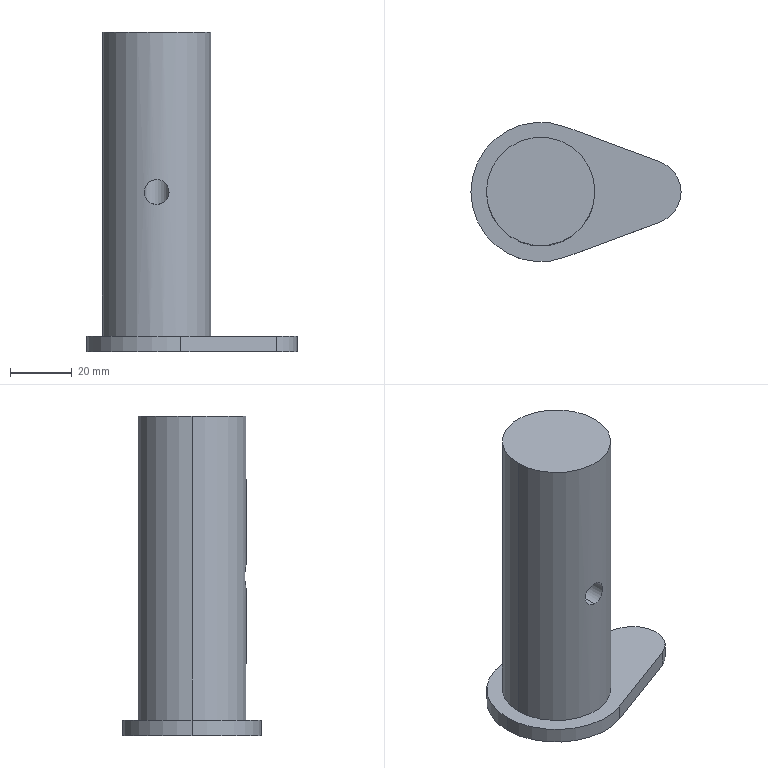Part | SolidWorks | features ICE 3, Extrusion 1 | 1 solid | 16 faces | box 67.801 x 45 x 103 mm | volume 100967 mm3 | cylinder 10 | plane 6 | commonest cylinder face diameters 8 x5 35 x2 45 x2 20.602 x1
STEP:
#1=CARTESIAN_POINT('',(0.,-17.5,47.5));
#2=VERTEX_POINT('',#1);
#3=CARTESIAN_POINT('',(0.,-17.5,55.5));
#4=VERTEX_POINT('',#3);
#5=CARTESIAN_POINT('',(0.,-17.5,47.5));
#6=CARTESIAN_POINT('',(-0.2615,-17.5,47.5));
#7=CARTESIAN_POINT('',(-0.522,-17.494,47.525));
#8=CARTESIAN_POINT('',(-1.041,-17.471,47.629));
#9=CARTESIAN_POINT('',(-1.292,-17.454,47.705));
#10=CARTESIAN_POINT('',(-1.773,-17.412,47.905));
#11=CARTESIAN_POINT('',(-2.007,-17.386,48.03));
#12=CARTESIAN_POINT('',(-2.442,-17.33,48.321));
#13=CARTESIAN_POINT('',(-2.643,-17.3,48.486));
#14=CARTESIAN_POINT('',(-3.012,-17.24,48.854));
#15=CARTESIAN_POINT('',(-3.18,-17.209,49.059));
#16=CARTESIAN_POINT('',(-3.469,-17.153,49.492));
#17=CARTESIAN_POINT('',(-3.592,-17.128,49.721));
#18=CARTESIAN_POINT('',(-3.794,-17.084,50.207));
#19=CARTESIAN_POINT('',(-3.871,-17.067,50.459));
#20=CARTESIAN_POINT('',(-3.973,-17.043,50.971));
#21=CARTESIAN_POINT('',(-4.,-17.037,51.234));
#22=CARTESIAN_POINT('',(-4.,-17.037,51.762));
#23=CARTESIAN_POINT('',(-3.974,-17.043,52.023));
#24=CARTESIAN_POINT('',(-3.872,-17.066,52.536));
#25=CARTESIAN_POINT('',(-3.795,-17.084,52.791));
#26=CARTESIAN_POINT('',(-3.595,-17.127,53.274));
#27=CARTESIAN_POINT('',(-3.472,-17.153,53.503));
#28=CARTESIAN_POINT('',(-3.181,-17.209,53.939));
#29=CARTESIAN_POINT('',(-3.014,-17.24,54.143));
#30=CARTESIAN_POINT('',(-2.647,-17.3,54.51));
#31=CARTESIAN_POINT('',(-2.444,-17.33,54.677));
#32=CARTESIAN_POINT('',(-2.008,-17.386,54.97));
#33=CARTESIAN_POINT('',(-1.778,-17.411,55.093));
#34=CARTESIAN_POINT('',(-1.297,-17.454,55.293));
#35=CARTESIAN_POINT('',(-1.042,-17.471,55.371));
#36=CARTESIAN_POINT('',(-0.5267,-17.494,55.474));
#37=CARTESIAN_POINT('',(-0.2652,-17.5,55.5));
#38=CARTESIAN_POINT('',(0.,-17.5,55.5));
#39=B_SPLINE_CURVE_WITH_KNOTS('',3,(#5,#6,#7,#8,#9,#10,#11,#12,#13,#14,#15,#16,#17,#18,#19,#20,#21,#22,#23,#24,#25,#26,#27,#28,#29,#30,#31,#32,#33,#34,#35,#36,#37,#38),.UNSPECIFIED.,.F.,.F.,(4,2,2,2,2,2,2,2,2,2,2,2,2,2,2,2,4),(0.01255,0.01333,0.01412,0.0149,0.01568,0.01647,0.01725,0.01804,0.01882,0.0196,0.02039,0.02117,0.02196,0.02274,0.02352,0.02431,0.02509),.UNSPECIFIED.);
#40=EDGE_CURVE('',#2,#4,#39,.T.);
#41=ORIENTED_EDGE('',*,*,#40,.F.);
#42=CARTESIAN_POINT('',(0.,-4.,47.5));
#43=VERTEX_POINT('',#42);
#44=CARTESIAN_POINT('',(0.,-70.,47.5));
#45=DIRECTION('',(0.,1.,0.));
#46=VECTOR('',#45,1000.);
#47=LINE('',#44,#46);
#48=EDGE_CURVE('',#2,#43,#47,.T.);
#49=ORIENTED_EDGE('',*,*,#48,.T.);
#50=CARTESIAN_POINT('',(-4.,0.,51.5));
#51=VERTEX_POINT('',#50);
#52=CARTESIAN_POINT('',(-4.,0.,51.5));
#53=CARTESIAN_POINT('',(-4.,-2.343,49.157));
#54=CARTESIAN_POINT('',(-2.343,-4.,47.5));
#55=CARTESIAN_POINT('',(0.,-4.,47.5));
#56=(BOUNDED_CURVE()B_SPLINE_CURVE(3,(#52,#53,#54,#55),.UNSPECIFIED.,.F.,.F.)B_SPLINE_CURVE_WITH_KNOTS((4,4),(4.712,6.283),.UNSPECIFIED.)CURVE()GEOMETRIC_REPRESENTATION_ITEM()RATIONAL_B_SPLINE_CURVE((1.,0.8047,0.8047,1.))REPRESENTATION_ITEM(''));
#57=EDGE_CURVE('',#51,#43,#56,.T.);
#58=ORIENTED_EDGE('',*,*,#57,.F.);
#59=CARTESIAN_POINT('',(0.,-4.,55.5));
#60=VERTEX_POINT('',#59);
#61=CARTESIAN_POINT('',(0.,-4.,55.5));
#62=CARTESIAN_POINT('',(-2.343,-4.,55.5));
#63=CARTESIAN_POINT('',(-4.,-2.343,53.843));
#64=CARTESIAN_POINT('',(-4.,0.,51.5));
#65=(BOUNDED_CURVE()B_SPLINE_CURVE(3,(#61,#62,#63,#64),.UNSPECIFIED.,.F.,.T.)B_SPLINE_CURVE_WITH_KNOTS((4,4),(3.142,4.712),.UNSPECIFIED.)CURVE()GEOMETRIC_REPRESENTATION_ITEM()RATIONAL_B_SPLINE_CURVE((1.,0.8047,0.8047,1.))REPRESENTATION_ITEM(''));
#66=EDGE_CURVE('',#60,#51,#65,.T.);
#67=ORIENTED_EDGE('',*,*,#66,.F.);
#68=CARTESIAN_POINT('',(0.,-70.,55.5));
#69=DIRECTION('',(0.,1.,0.));
#70=VECTOR('',#69,1000.);
#71=LINE('',#68,#70);
#72=EDGE_CURVE('',#4,#60,#71,.T.);
#73=ORIENTED_EDGE('',*,*,#72,.F.);
#74=EDGE_LOOP('',(#41,#49,#58,#67,#73));
#75=FACE_OUTER_BOUND('',#74,.T.);
#76=CARTESIAN_POINT('',(0.,-70.,51.5));
#77=DIRECTION('',(0.,1.,0.));
#78=DIRECTION('',(0.,0.,1.));
#79=AXIS2_PLACEMENT_3D('',#76,#77,#78);
#80=CYLINDRICAL_SURFACE('',#79,4.);
#81=ADVANCED_FACE('',(#75),#80,.F.);
#82=CARTESIAN_POINT('',(4.,0.,70.));
#83=VERTEX_POINT('',#82);
#84=CARTESIAN_POINT('',(-4.,0.,70.));
#85=VERTEX_POINT('',#84);
#86=CARTESIAN_POINT('',(0.,0.,70.));
#87=DIRECTION('',(0.,0.,-1.));
#88=DIRECTION('',(-1.,0.,0.));
#89=AXIS2_PLACEMENT_3D('',#86,#87,#88);
#90=CIRCLE('',#89,4.);
#91=EDGE_CURVE('',#83,#85,#90,.T.);
#92=ORIENTED_EDGE('',*,*,#91,.F.);
#93=CARTESIAN_POINT('',(4.,0.,51.5));
#94=VERTEX_POINT('',#93);
#95=CARTESIAN_POINT('',(4.,0.,70.));
#96=DIRECTION('',(0.,0.,-1.));
#97=VECTOR('',#96,1000.);
#98=LINE('',#95,#97);
#99=EDGE_CURVE('',#83,#94,#98,.T.);
#100=ORIENTED_EDGE('',*,*,#99,.T.);
#101=CARTESIAN_POINT('',(4.,0.,51.5));
#102=CARTESIAN_POINT('',(4.,-2.343,53.843));
#103=CARTESIAN_POINT('',(2.343,-4.,55.5));
#104=CARTESIAN_POINT('',(0.,-4.,55.5));
#105=(BOUNDED_CURVE()B_SPLINE_CURVE(3,(#101,#102,#103,#104),.UNSPECIFIED.,.F.,.T.)B_SPLINE_CURVE_WITH_KNOTS((4,4),(1.571,3.142),.UNSPECIFIED.)CURVE()GEOMETRIC_REPRESENTATION_ITEM()RATIONAL_B_SPLINE_CURVE((1.,0.8047,0.8047,1.))REPRESENTATION_ITEM(''));
#106=EDGE_CURVE('',#94,#60,#105,.T.);
#107=ORIENTED_EDGE('',*,*,#106,.T.);
#108=ORIENTED_EDGE('',*,*,#66,.T.);
#109=CARTESIAN_POINT('',(-4.,0.,70.));
#110=DIRECTION('',(0.,0.,-1.));
#111=VECTOR('',#110,1000.);
#112=LINE('',#109,#111);
#113=EDGE_CURVE('',#85,#51,#112,.T.);
#114=ORIENTED_EDGE('',*,*,#113,.F.);
#115=EDGE_LOOP('',(#92,#100,#107,#108,#114));
#116=FACE_OUTER_BOUND('',#115,.T.);
#117=CARTESIAN_POINT('',(0.,0.,70.));
#118=DIRECTION('',(0.,0.,-1.));
#119=DIRECTION('',(-1.,0.,0.));
#120=AXIS2_PLACEMENT_3D('',#117,#118,#119);
#121=CYLINDRICAL_SURFACE('',#120,4.);
#122=ADVANCED_FACE('',(#116),#121,.F.);
#123=ORIENTED_EDGE('',*,*,#57,.T.);
#124=CARTESIAN_POINT('',(0.,-4.,47.5));
#125=CARTESIAN_POINT('',(2.343,-4.,47.5));
#126=CARTESIAN_POINT('',(4.,-2.343,49.157));
#127=CARTESIAN_POINT('',(4.,0.,51.5));
#128=(BOUNDED_CURVE()B_SPLINE_CURVE(3,(#124,#125,#126,#127),.UNSPECIFIED.,.F.,.F.)B_SPLINE_CURVE_WITH_KNOTS((4,4),(0.,1.571),.UNSPECIFIED.)CURVE()GEOMETRIC_REPRESENTATION_ITEM()RATIONAL_B_SPLINE_CURVE((1.,0.8047,0.8047,1.))REPRESENTATION_ITEM(''));
#129=EDGE_CURVE('',#43,#94,#128,.T.);
#130=ORIENTED_EDGE('',*,*,#129,.T.);
#131=CARTESIAN_POINT('',(4.,0.,0.));
#132=VERTEX_POINT('',#131);
#133=CARTESIAN_POINT('',(4.,0.,70.));
#134=DIRECTION('',(0.,0.,-1.));
#135=VECTOR('',#134,1000.);
#136=LINE('',#133,#135);
#137=EDGE_CURVE('',#94,#132,#136,.T.);
#138=ORIENTED_EDGE('',*,*,#137,.T.);
#139=CARTESIAN_POINT('',(-4.,0.,0.));
#140=VERTEX_POINT('',#139);
#141=CARTESIAN_POINT('',(0.,0.,0.));
#142=DIRECTION('',(0.,0.,-1.));
#143=DIRECTION('',(-1.,0.,0.));
#144=AXIS2_PLACEMENT_3D('',#141,#142,#143);
#145=CIRCLE('',#144,4.);
#146=EDGE_CURVE('',#132,#140,#145,.T.);
#147=ORIENTED_EDGE('',*,*,#146,.T.);
#148=CARTESIAN_POINT('',(-4.,0.,70.));
#149=DIRECTION('',(0.,0.,-1.));
#150=VECTOR('',#149,1000.);
#151=LINE('',#148,#150);
#152=EDGE_CURVE('',#51,#140,#151,.T.);
#153=ORIENTED_EDGE('',*,*,#152,.F.);
#154=EDGE_LOOP('',(#123,#130,#138,#147,#153));
#155=FACE_OUTER_BOUND('',#154,.T.);
#156=CARTESIAN_POINT('',(0.,0.,70.));
#157=DIRECTION('',(0.,0.,-1.));
#158=DIRECTION('',(-1.,0.,0.));
#159=AXIS2_PLACEMENT_3D('',#156,#157,#158);
#160=CYLINDRICAL_SURFACE('',#159,4.);
#161=ADVANCED_FACE('',(#155),#160,.F.);
#162=CARTESIAN_POINT('',(7.842,-21.089,5.));
#163=VERTEX_POINT('',#162);
#164=CARTESIAN_POINT('',(-22.5,0.,5.));
#165=VERTEX_POINT('',#164);
#166=CARTESIAN_POINT('',(0.,0.,5.));
#167=DIRECTION('',(0.,0.,-1.));
#168=DIRECTION('',(-1.,0.,0.));
#169=AXIS2_PLACEMENT_3D('',#166,#167,#168);
#170=CIRCLE('',#169,22.5);
#171=EDGE_CURVE('',#163,#165,#170,.T.);
#172=ORIENTED_EDGE('',*,*,#171,.T.);
#173=CARTESIAN_POINT('',(-22.5,0.,0.));
#174=VERTEX_POINT('',#173);
#175=CARTESIAN_POINT('',(-22.5,0.,5.));
#176=DIRECTION('',(0.,0.,-1.));
#177=VECTOR('',#176,1000.);
#178=LINE('',#175,#177);
#179=EDGE_CURVE('',#165,#174,#178,.T.);
#180=ORIENTED_EDGE('',*,*,#179,.T.);
#181=CARTESIAN_POINT('',(7.842,-21.089,0.));
#182=VERTEX_POINT('',#181);
#183=CARTESIAN_POINT('',(0.,0.,0.));
#184=DIRECTION('',(0.,0.,-1.));
#185=DIRECTION('',(-1.,0.,0.));
#186=AXIS2_PLACEMENT_3D('',#183,#184,#185);
#187=CIRCLE('',#186,22.5);
#188=EDGE_CURVE('',#182,#174,#187,.T.);
#189=ORIENTED_EDGE('',*,*,#188,.F.);
#190=CARTESIAN_POINT('',(7.842,-21.089,5.));
#191=DIRECTION('',(0.,0.,-1.));
#192=VECTOR('',#191,1000.);
#193=LINE('',#190,#192);
#194=EDGE_CURVE('',#163,#182,#193,.T.);
#195=ORIENTED_EDGE('',*,*,#194,.F.);
#196=EDGE_LOOP('',(#172,#180,#189,#195));
#197=FACE_OUTER_BOUND('',#196,.T.);
#198=CARTESIAN_POINT('',(0.,0.,5.));
#199=DIRECTION('',(0.,0.,-1.));
#200=DIRECTION('',(-1.,0.,0.));
#201=AXIS2_PLACEMENT_3D('',#198,#199,#200);
#202=CYLINDRICAL_SURFACE('',#201,22.5);
#203=ADVANCED_FACE('',(#197),#202,.T.);
#204=CARTESIAN_POINT('',(17.5,0.,103.));
#205=VERTEX_POINT('',#204);
#206=CARTESIAN_POINT('',(-17.5,0.,103.));
#207=VERTEX_POINT('',#206);
#208=CARTESIAN_POINT('',(0.,0.,103.));
#209=DIRECTION('',(0.,0.,1.));
#210=DIRECTION('',(1.,0.,0.));
#211=AXIS2_PLACEMENT_3D('',#208,#209,#210);
#212=CIRCLE('',#211,17.5);
#213=EDGE_CURVE('',#205,#207,#212,.T.);
#214=ORIENTED_EDGE('',*,*,#213,.F.);
#215=CARTESIAN_POINT('',(17.5,0.,5.));
#216=VERTEX_POINT('',#215);
#217=CARTESIAN_POINT('',(17.5,0.,103.));
#218=DIRECTION('',(0.,0.,-1.));
#219=VECTOR('',#218,1000.);
#220=LINE('',#217,#219);
#221=EDGE_CURVE('',#205,#216,#220,.T.);
#222=ORIENTED_EDGE('',*,*,#221,.T.);
#223=CARTESIAN_POINT('',(-17.5,0.,5.));
#224=VERTEX_POINT('',#223);
#225=CARTESIAN_POINT('',(0.,0.,5.));
#226=DIRECTION('',(0.,0.,-1.));
#227=DIRECTION('',(-1.,0.,0.));
#228=AXIS2_PLACEMENT_3D('',#225,#226,#227);
#229=CIRCLE('',#228,17.5);
#230=EDGE_CURVE('',#224,#216,#229,.T.);
#231=ORIENTED_EDGE('',*,*,#230,.F.);
#232=CARTESIAN_POINT('',(-17.5,0.,103.));
#233=DIRECTION('',(0.,0.,-1.));
#234=VECTOR('',#233,1000.);
#235=LINE('',#232,#234);
#236=EDGE_CURVE('',#207,#224,#235,.T.);
#237=ORIENTED_EDGE('',*,*,#236,.F.);
#238=EDGE_LOOP('',(#214,#222,#231,#237));
#239=FACE_OUTER_BOUND('',#238,.T.);
#240=CARTESIAN_POINT('',(0.,0.,103.));
#241=DIRECTION('',(0.,0.,-1.));
#242=DIRECTION('',(-1.,0.,0.));
#243=AXIS2_PLACEMENT_3D('',#240,#241,#242);
#244=CYLINDRICAL_SURFACE('',#243,17.5);
#245=ADVANCED_FACE('',(#239),#244,.T.);
#246=ORIENTED_EDGE('',*,*,#221,.F.);
#247=CARTESIAN_POINT('',(0.,0.,103.));
#248=DIRECTION('',(0.,0.,1.));
#249=DIRECTION('',(1.,0.,0.));
#250=AXIS2_PLACEMENT_3D('',#247,#248,#249);
#251=CIRCLE('',#250,17.5);
#252=EDGE_CURVE('',#207,#205,#251,.T.);
#253=ORIENTED_EDGE('',*,*,#252,.F.);
#254=ORIENTED_EDGE('',*,*,#236,.T.);
#255=CARTESIAN_POINT('',(0.,0.,5.));
#256=DIRECTION('',(0.,0.,-1.));
#257=DIRECTION('',(-1.,0.,0.));
#258=AXIS2_PLACEMENT_3D('',#255,#256,#257);
#259=CIRCLE('',#258,17.5);
#260=EDGE_CURVE('',#216,#224,#259,.T.);
#261=ORIENTED_EDGE('',*,*,#260,.F.);
#262=EDGE_LOOP('',(#246,#253,#254,#261));
#263=FACE_OUTER_BOUND('',#262,.T.);
#264=CARTESIAN_POINT('',(0.,-17.5,55.5));
#265=CARTESIAN_POINT('',(0.2652,-17.5,55.5));
#266=CARTESIAN_POINT('',(0.5259,-17.494,55.474));
#267=CARTESIAN_POINT('',(1.038,-17.471,55.372));
#268=CARTESIAN_POINT('',(1.293,-17.454,55.294));
#269=CARTESIAN_POINT('',(1.777,-17.411,55.093));
#270=CARTESIAN_POINT('',(2.006,-17.386,54.97));
#271=CARTESIAN_POINT('',(2.441,-17.33,54.68));
#272=CARTESIAN_POINT('',(2.645,-17.3,54.512));
#273=CARTESIAN_POINT('',(3.013,-17.24,54.144));
#274=CARTESIAN_POINT('',(3.178,-17.21,53.943));
#275=CARTESIAN_POINT('',(3.471,-17.153,53.506));
#276=CARTESIAN_POINT('',(3.594,-17.127,53.274));
#277=CARTESIAN_POINT('',(3.794,-17.084,52.793));
#278=CARTESIAN_POINT('',(3.871,-17.067,52.54));
#279=CARTESIAN_POINT('',(3.974,-17.043,52.024));
#280=CARTESIAN_POINT('',(4.,-17.037,51.763));
#281=CARTESIAN_POINT('',(4.,-17.037,51.24));
#282=CARTESIAN_POINT('',(3.974,-17.043,50.974));
#283=CARTESIAN_POINT('',(3.871,-17.067,50.46));
#284=CARTESIAN_POINT('',(3.795,-17.084,50.21));
#285=CARTESIAN_POINT('',(3.594,-17.127,49.725));
#286=CARTESIAN_POINT('',(3.469,-17.153,49.492));
#287=CARTESIAN_POINT('',(3.18,-17.209,49.06));
#288=CARTESIAN_POINT('',(3.014,-17.24,48.857));
#289=CARTESIAN_POINT('',(2.642,-17.3,48.486));
#290=CARTESIAN_POINT('',(2.441,-17.33,48.321));
#291=CARTESIAN_POINT('',(2.009,-17.386,48.031));
#292=CARTESIAN_POINT('',(1.774,-17.411,47.906));
#293=CARTESIAN_POINT('',(1.291,-17.454,47.705));
#294=CARTESIAN_POINT('',(1.042,-17.471,47.629));
#295=CARTESIAN_POINT('',(0.5271,-17.494,47.526));
#296=CARTESIAN_POINT('',(0.2616,-17.5,47.5));
#297=CARTESIAN_POINT('',(0.,-17.5,47.5));
#298=B_SPLINE_CURVE_WITH_KNOTS('',3,(#264,#265,#266,#267,#268,#269,#270,#271,#272,#273,#274,#275,#276,#277,#278,#279,#280,#281,#282,#283,#284,#285,#286,#287,#288,#289,#290,#291,#292,#293,#294,#295,#296,#297),.UNSPECIFIED.,.F.,.F.,(4,2,2,2,2,2,2,2,2,2,2,2,2,2,2,2,4),(0.,0.0007842,0.001568,0.002353,0.003137,0.003921,0.004705,0.005489,0.006274,0.007058,0.007842,0.008626,0.009411,0.01019,0.01098,0.01176,0.01255),.UNSPECIFIED.);
#299=EDGE_CURVE('',#4,#2,#298,.T.);
#300=ORIENTED_EDGE('',*,*,#299,.T.);
#301=ORIENTED_EDGE('',*,*,#40,.T.);
#302=EDGE_LOOP('',(#300,#301));
#303=FACE_BOUND('',#302,.T.);
#304=CARTESIAN_POINT('',(0.,0.,103.));
#305=DIRECTION('',(0.,0.,-1.));
#306=DIRECTION('',(-1.,0.,0.));
#307=AXIS2_PLACEMENT_3D('',#304,#305,#306);
#308=CYLINDRICAL_SURFACE('',#307,17.5);
#309=ADVANCED_FACE('',(#263,#303),#308,.T.);
#310=ORIENTED_EDGE('',*,*,#252,.T.);
#311=ORIENTED_EDGE('',*,*,#213,.T.);
#312=EDGE_LOOP('',(#310,#311));
#313=FACE_OUTER_BOUND('',#312,.T.);
#314=CARTESIAN_POINT('',(0.,0.,103.));
#315=DIRECTION('',(0.,0.,1.));
#316=DIRECTION('',(1.,0.,0.));
#317=AXIS2_PLACEMENT_3D('',#314,#315,#316);
#318=PLANE('',#317);
#319=ADVANCED_FACE('',(#313),#318,.T.);
#320=CARTESIAN_POINT('',(38.59,-9.655,5.));
#321=VERTEX_POINT('',#320);
#322=CARTESIAN_POINT('',(7.842,-21.089,5.));
#323=DIRECTION('',(-0.9373,-0.3485,0.));
#324=VECTOR('',#323,1000.);
#325=LINE('',#322,#324);
#326=EDGE_CURVE('',#321,#163,#325,.T.);
#327=ORIENTED_EDGE('',*,*,#326,.F.);
#328=CARTESIAN_POINT('',(38.59,9.655,5.));
#329=VERTEX_POINT('',#328);
#330=CARTESIAN_POINT('',(35.,0.,5.));
#331=DIRECTION('',(0.,0.,-1.));
#332=DIRECTION('',(-1.,0.,0.));
#333=AXIS2_PLACEMENT_3D('',#330,#331,#332);
#334=CIRCLE('',#333,10.301);
#335=EDGE_CURVE('',#329,#321,#334,.T.);
#336=ORIENTED_EDGE('',*,*,#335,.F.);
#337=CARTESIAN_POINT('',(7.842,21.089,5.));
#338=VERTEX_POINT('',#337);
#339=CARTESIAN_POINT('',(7.842,21.089,5.));
#340=DIRECTION('',(-0.9373,0.3485,0.));
#341=VECTOR('',#340,1000.);
#342=LINE('',#339,#341);
#343=EDGE_CURVE('',#329,#338,#342,.T.);
#344=ORIENTED_EDGE('',*,*,#343,.T.);
#345=CARTESIAN_POINT('',(0.,0.,5.));
#346=DIRECTION('',(0.,0.,-1.));
#347=DIRECTION('',(-1.,0.,0.));
#348=AXIS2_PLACEMENT_3D('',#345,#346,#347);
#349=CIRCLE('',#348,22.5);
#350=EDGE_CURVE('',#165,#338,#349,.T.);
#351=ORIENTED_EDGE('',*,*,#350,.F.);
#352=ORIENTED_EDGE('',*,*,#171,.F.);
#353=EDGE_LOOP('',(#327,#336,#344,#351,#352));
#354=FACE_OUTER_BOUND('',#353,.T.);
#355=ORIENTED_EDGE('',*,*,#230,.T.);
#356=ORIENTED_EDGE('',*,*,#260,.T.);
#357=EDGE_LOOP('',(#355,#356));
#358=FACE_BOUND('',#357,.T.);
#359=CARTESIAN_POINT('',(0.,0.,5.));
#360=DIRECTION('',(0.,0.,-1.));
#361=DIRECTION('',(-1.,0.,0.));
#362=AXIS2_PLACEMENT_3D('',#359,#360,#361);
#363=PLANE('',#362);
#364=ADVANCED_FACE('',(#354,#358),#363,.F.);
#365=CARTESIAN_POINT('',(38.59,-9.655,0.));
#366=VERTEX_POINT('',#365);
#367=CARTESIAN_POINT('',(7.842,-21.089,0.));
#368=DIRECTION('',(-0.9373,-0.3485,0.));
#369=VECTOR('',#368,1000.);
#370=LINE('',#367,#369);
#371=EDGE_CURVE('',#366,#182,#370,.T.);
#372=ORIENTED_EDGE('',*,*,#371,.F.);
#373=CARTESIAN_POINT('',(38.59,-9.655,5.));
#374=DIRECTION('',(0.,0.,-1.));
#375=VECTOR('',#374,1000.);
#376=LINE('',#373,#375);
#377=EDGE_CURVE('',#321,#366,#376,.T.);
#378=ORIENTED_EDGE('',*,*,#377,.F.);
#379=ORIENTED_EDGE('',*,*,#326,.T.);
#380=ORIENTED_EDGE('',*,*,#194,.T.);
#381=EDGE_LOOP('',(#372,#378,#379,#380));
#382=FACE_OUTER_BOUND('',#381,.T.);
#383=CARTESIAN_POINT('',(7.842,-21.089,5.));
#384=DIRECTION('',(0.3485,-0.9373,0.));
#385=DIRECTION('',(0.9373,0.3485,0.));
#386=AXIS2_PLACEMENT_3D('',#383,#384,#385);
#387=PLANE('',#386);
#388=ADVANCED_FACE('',(#382),#387,.T.);
#389=CARTESIAN_POINT('',(38.59,9.655,0.));
#390=VERTEX_POINT('',#389);
#391=CARTESIAN_POINT('',(35.,0.,0.));
#392=DIRECTION('',(0.,0.,-1.));
#393=DIRECTION('',(-1.,0.,0.));
#394=AXIS2_PLACEMENT_3D('',#391,#392,#393);
#395=CIRCLE('',#394,10.301);
#396=EDGE_CURVE('',#390,#366,#395,.T.);
#397=ORIENTED_EDGE('',*,*,#396,.F.);
#398=CARTESIAN_POINT('',(38.59,9.655,5.));
#399=DIRECTION('',(0.,0.,-1.));
#400=VECTOR('',#399,1000.);
#401=LINE('',#398,#400);
#402=EDGE_CURVE('',#329,#390,#401,.T.);
#403=ORIENTED_EDGE('',*,*,#402,.F.);
#404=ORIENTED_EDGE('',*,*,#335,.T.);
#405=ORIENTED_EDGE('',*,*,#377,.T.);
#406=EDGE_LOOP('',(#397,#403,#404,#405));
#407=FACE_OUTER_BOUND('',#406,.T.);
#408=CARTESIAN_POINT('',(35.,0.,5.));
#409=DIRECTION('',(0.,0.,-1.));
#410=DIRECTION('',(-1.,0.,0.));
#411=AXIS2_PLACEMENT_3D('',#408,#409,#410);
#412=CYLINDRICAL_SURFACE('',#411,10.301);
#413=ADVANCED_FACE('',(#407),#412,.T.);
#414=CARTESIAN_POINT('',(7.842,21.089,0.));
#415=VERTEX_POINT('',#414);
#416=CARTESIAN_POINT('',(7.842,21.089,0.));
#417=DIRECTION('',(-0.9373,0.3485,0.));
#418=VECTOR('',#417,1000.);
#419=LINE('',#416,#418);
#420=EDGE_CURVE('',#390,#415,#419,.T.);
#421=ORIENTED_EDGE('',*,*,#420,.T.);
#422=CARTESIAN_POINT('',(7.842,21.089,5.));
#423=DIRECTION('',(0.,0.,-1.));
#424=VECTOR('',#423,1000.);
#425=LINE('',#422,#424);
#426=EDGE_CURVE('',#338,#415,#425,.T.);
#427=ORIENTED_EDGE('',*,*,#426,.F.);
#428=ORIENTED_EDGE('',*,*,#343,.F.);
#429=ORIENTED_EDGE('',*,*,#402,.T.);
#430=EDGE_LOOP('',(#421,#427,#428,#429));
#431=FACE_OUTER_BOUND('',#430,.T.);
#432=CARTESIAN_POINT('',(7.842,21.089,5.));
#433=DIRECTION('',(-0.3485,-0.9373,0.));
#434=DIRECTION('',(0.9373,-0.3485,0.));
#435=AXIS2_PLACEMENT_3D('',#432,#433,#434);
#436=PLANE('',#435);
#437=ADVANCED_FACE('',(#431),#436,.F.);
#438=ORIENTED_EDGE('',*,*,#179,.F.);
#439=ORIENTED_EDGE('',*,*,#350,.T.);
#440=ORIENTED_EDGE('',*,*,#426,.T.);
#441=CARTESIAN_POINT('',(0.,0.,0.));
#442=DIRECTION('',(0.,0.,-1.));
#443=DIRECTION('',(-1.,0.,0.));
#444=AXIS2_PLACEMENT_3D('',#441,#442,#443);
#445=CIRCLE('',#444,22.5);
#446=EDGE_CURVE('',#174,#415,#445,.T.);
#447=ORIENTED_EDGE('',*,*,#446,.F.);
#448=EDGE_LOOP('',(#438,#439,#440,#447));
#449=FACE_OUTER_BOUND('',#448,.T.);
#450=CARTESIAN_POINT('',(0.,0.,5.));
#451=DIRECTION('',(0.,0.,-1.));
#452=DIRECTION('',(-1.,0.,0.));
#453=AXIS2_PLACEMENT_3D('',#450,#451,#452);
#454=CYLINDRICAL_SURFACE('',#453,22.5);
#455=ADVANCED_FACE('',(#449),#454,.T.);
#456=CARTESIAN_POINT('',(0.,0.,0.));
#457=DIRECTION('',(0.,0.,-1.));
#458=DIRECTION('',(-1.,0.,0.));
#459=AXIS2_PLACEMENT_3D('',#456,#457,#458);
#460=CIRCLE('',#459,4.);
#461=EDGE_CURVE('',#140,#132,#460,.T.);
#462=ORIENTED_EDGE('',*,*,#461,.F.);
#463=ORIENTED_EDGE('',*,*,#146,.F.);
#464=EDGE_LOOP('',(#462,#463));
#465=FACE_BOUND('',#464,.T.);
#466=ORIENTED_EDGE('',*,*,#371,.T.);
#467=ORIENTED_EDGE('',*,*,#188,.T.);
#468=ORIENTED_EDGE('',*,*,#446,.T.);
#469=ORIENTED_EDGE('',*,*,#420,.F.);
#470=ORIENTED_EDGE('',*,*,#396,.T.);
#471=EDGE_LOOP('',(#466,#467,#468,#469,#470));
#472=FACE_OUTER_BOUND('',#471,.T.);
#473=CARTESIAN_POINT('',(0.,0.,0.));
#474=DIRECTION('',(0.,0.,1.));
#475=DIRECTION('',(1.,0.,0.));
#476=AXIS2_PLACEMENT_3D('',#473,#474,#475);
#477=PLANE('',#476);
#478=ADVANCED_FACE('',(#465,#472),#477,.F.);
#479=ORIENTED_EDGE('',*,*,#99,.F.);
#480=CARTESIAN_POINT('',(0.,0.,70.));
#481=DIRECTION('',(0.,0.,-1.));
#482=DIRECTION('',(-1.,0.,0.));
#483=AXIS2_PLACEMENT_3D('',#480,#481,#482);
#484=CIRCLE('',#483,4.);
#485=EDGE_CURVE('',#85,#83,#484,.T.);
#486=ORIENTED_EDGE('',*,*,#485,.F.);
#487=ORIENTED_EDGE('',*,*,#113,.T.);
#488=ORIENTED_EDGE('',*,*,#152,.T.);
#489=ORIENTED_EDGE('',*,*,#461,.T.);
#490=ORIENTED_EDGE('',*,*,#137,.F.);
#491=EDGE_LOOP('',(#479,#486,#487,#488,#489,#490));
#492=FACE_OUTER_BOUND('',#491,.T.);
#493=CARTESIAN_POINT('',(0.,0.,70.));
#494=DIRECTION('',(0.,0.,-1.));
#495=DIRECTION('',(-1.,0.,0.));
#496=AXIS2_PLACEMENT_3D('',#493,#494,#495);
#497=CYLINDRICAL_SURFACE('',#496,4.);
#498=ADVANCED_FACE('',(#492),#497,.F.);
#499=ORIENTED_EDGE('',*,*,#485,.T.);
#500=ORIENTED_EDGE('',*,*,#91,.T.);
#501=EDGE_LOOP('',(#499,#500));
#502=FACE_OUTER_BOUND('',#501,.T.);
#503=CARTESIAN_POINT('',(0.,0.,70.));
#504=DIRECTION('',(0.,0.,-1.));
#505=DIRECTION('',(-1.,0.,0.));
#506=AXIS2_PLACEMENT_3D('',#503,#504,#505);
#507=PLANE('',#506);
#508=ADVANCED_FACE('',(#502),#507,.T.);
#509=ORIENTED_EDGE('',*,*,#48,.F.);
#510=ORIENTED_EDGE('',*,*,#299,.F.);
#511=ORIENTED_EDGE('',*,*,#72,.T.);
#512=ORIENTED_EDGE('',*,*,#106,.F.);
#513=ORIENTED_EDGE('',*,*,#129,.F.);
#514=EDGE_LOOP('',(#509,#510,#511,#512,#513));
#515=FACE_OUTER_BOUND('',#514,.T.);
#516=CARTESIAN_POINT('',(0.,-70.,51.5));
#517=DIRECTION('',(0.,1.,0.));
#518=DIRECTION('',(0.,0.,1.));
#519=AXIS2_PLACEMENT_3D('',#516,#517,#518);
#520=CYLINDRICAL_SURFACE('',#519,4.);
#521=ADVANCED_FACE('',(#515),#520,.F.);
#522=CLOSED_SHELL('',(#81,#122,#161,#203,#245,#309,#319,#364,#388,#413,#437,#455,#478,#498,#508,#521));
#523=MANIFOLD_SOLID_BREP('',#522);
#524=CARTESIAN_POINT('',(0.,0.,0.));
#525=DIRECTION('',(0.,0.,1.));
#526=DIRECTION('',(1.,0.,0.));
#527=AXIS2_PLACEMENT_3D('',#524,#525,#526);
#528=(LENGTH_UNIT()NAMED_UNIT(*)SI_UNIT(.MILLI.,.METRE.));
#529=UNCERTAINTY_MEASURE_WITH_UNIT(LENGTH_MEASURE(0.00001),#528,'','');
#530=(NAMED_UNIT(*)PLANE_ANGLE_UNIT()SI_UNIT($,.RADIAN.));
#531=(NAMED_UNIT(*)SI_UNIT($,.STERADIAN.)SOLID_ANGLE_UNIT());
#532=(GEOMETRIC_REPRESENTATION_CONTEXT(3)GLOBAL_UNCERTAINTY_ASSIGNED_CONTEXT((#529))GLOBAL_UNIT_ASSIGNED_CONTEXT((#528,#530,#531))REPRESENTATION_CONTEXT('',''));
#533=ADVANCED_BREP_SHAPE_REPRESENTATION('',(#523,#527),#532);